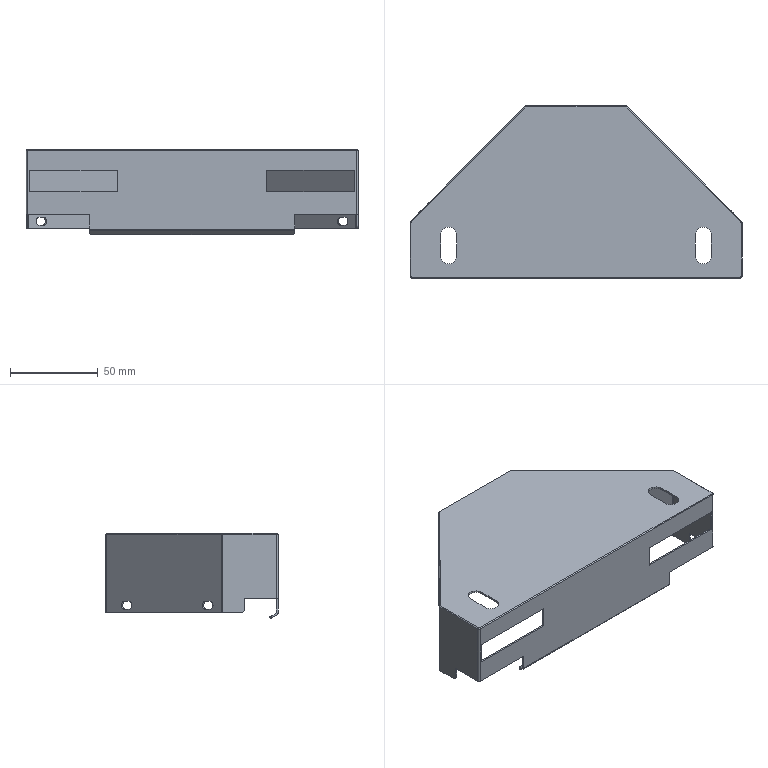Part | SolidWorks | features ICE 5, Chamfer 2, Fillet 2, BossThin 1, FlatPattern 1, MirrorPattern 1, SMBaseFlange 1, SheetMetal 1, Shell 1 | 1 solid | 98 faces | box 189 x 98 x 48.5 mm | volume 32493 mm3 | plane 56 | cylinder 36 | cone 6 | commonest cylinder face diameters 2 x14 4.5 x12 4 x6 9 x4